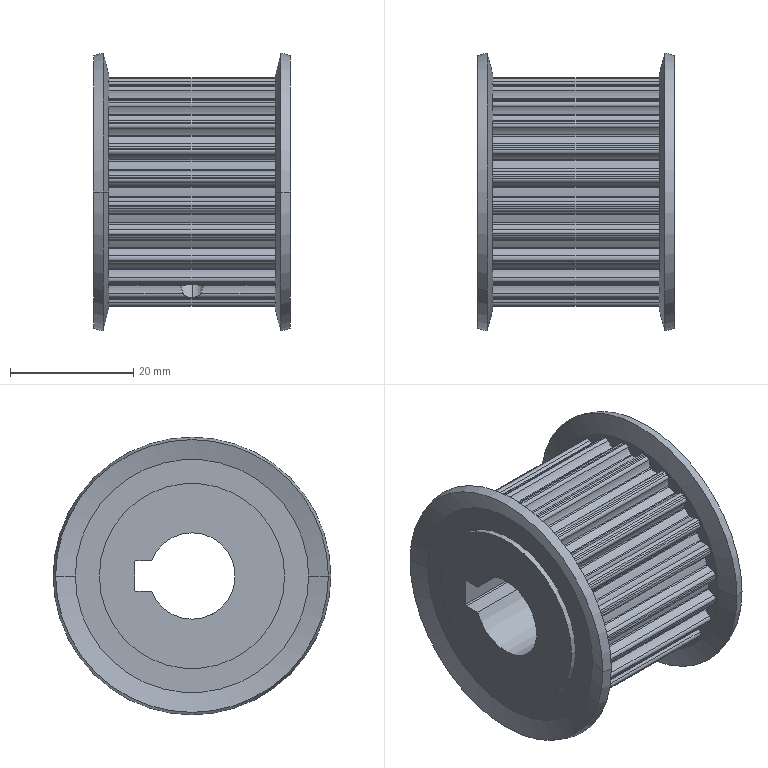Part | NX | 1 solid | 258 faces | box 32 x 45 x 45 mm | volume 27096 mm3 | cylinder 237 | cone 12 | plane 9 | commonest cylinder face diameters 0.5 x52 6.55 x52 1.1 x48 37.24 x48 33.7 x26 4.134 x4